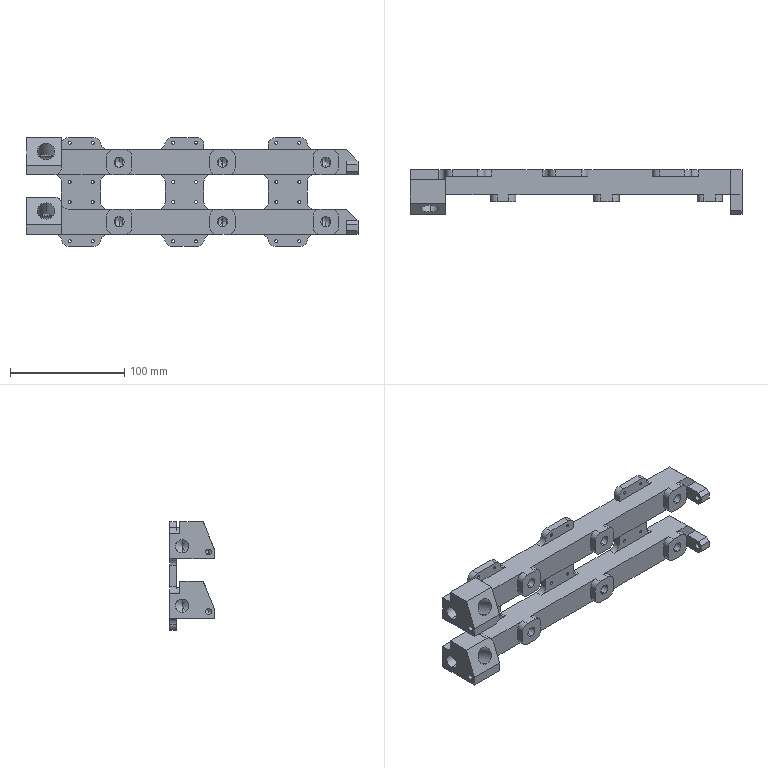NC program | NX | posted by the shop | part box 290 x 39.082 x 95 mm
Lines 1 to 25 of 5678:
(Created by : ADMINISTRATOR                           )
(零件名称            : 3978960 - MAINBOARD COOLING MANIFOLD SHO)
N10 G17 G21 G94 G90
(Zigzag-Face, tool: D63R0.8)
N12 T00 M6
N14 G54
N16 G17 G0 G90 X182.8 Y-31.75 S3000 M3
N18 G43 Z30. H0
N20 Z3.
N22 G94 G1 Z0. F1000.
N24 X176.5
N26 X-164.195
N28 G2 X-176.5 Y-19.445 R12.305
N30 X-161.46 Y-4.405 R15.04
N32 G1 X164.195
N34 G3 X176.5 Y7.9 R12.305
N36 X161.46 Y22.94 R15.04
N38 G1 X-176.5
N40 X-182.8
N42 Z3.
N44 G0 Z30.
N46 M5